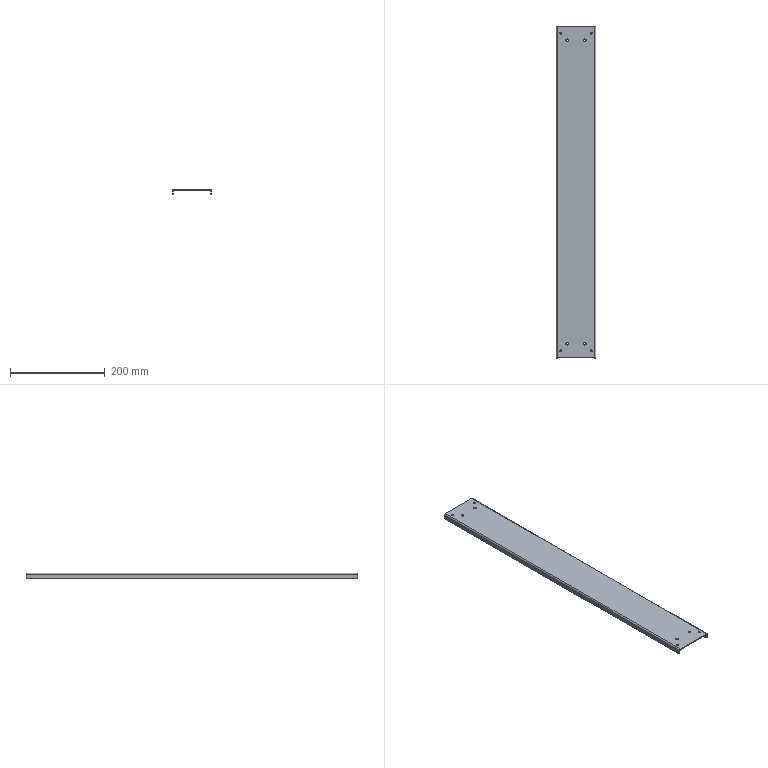Part | SolidWorks | features HoleWzd 3, Fillet 1, FlatPattern 1, SMBaseFlange 1, SheetMetal 1 | 1 solid | 42 faces | box 84 x 700 x 12 mm | volume 143164 mm3 | cylinder 24 | plane 18 | commonest cylinder face diameters 5.5 x10 4.5 x8 6 x4 1.5 x2
STEP:
#1=CARTESIAN_POINT('',(61.25,30.,2.));
#2=VERTEX_POINT('',#1);
#3=CARTESIAN_POINT('',(55.75,30.,2.));
#4=VERTEX_POINT('',#3);
#5=CARTESIAN_POINT('',(58.5,30.,2.));
#6=DIRECTION('',(0.,0.,-1.));
#7=DIRECTION('',(-1.,0.,0.));
#8=AXIS2_PLACEMENT_3D('',#5,#6,#7);
#9=CIRCLE('',#8,2.75);
#10=EDGE_CURVE('',#2,#4,#9,.T.);
#11=ORIENTED_EDGE('',*,*,#10,.F.);
#12=CARTESIAN_POINT('',(61.25,30.,0.));
#13=VERTEX_POINT('',#12);
#14=CARTESIAN_POINT('',(61.25,30.,0.));
#15=DIRECTION('',(0.,0.,-1.));
#16=VECTOR('',#15,1000.);
#17=LINE('',#14,#16);
#18=EDGE_CURVE('',#2,#13,#17,.T.);
#19=ORIENTED_EDGE('',*,*,#18,.T.);
#20=CARTESIAN_POINT('',(55.75,30.,0.));
#21=VERTEX_POINT('',#20);
#22=CARTESIAN_POINT('',(58.5,30.,0.));
#23=DIRECTION('',(0.,0.,-1.));
#24=DIRECTION('',(-1.,0.,0.));
#25=AXIS2_PLACEMENT_3D('',#22,#23,#24);
#26=CIRCLE('',#25,2.75);
#27=EDGE_CURVE('',#13,#21,#26,.T.);
#28=ORIENTED_EDGE('',*,*,#27,.T.);
#29=CARTESIAN_POINT('',(55.75,30.,0.));
#30=DIRECTION('',(0.,0.,-1.));
#31=VECTOR('',#30,1000.);
#32=LINE('',#29,#31);
#33=EDGE_CURVE('',#4,#21,#32,.T.);
#34=ORIENTED_EDGE('',*,*,#33,.F.);
#35=EDGE_LOOP('',(#11,#19,#28,#34));
#36=FACE_OUTER_BOUND('',#35,.T.);
#37=CARTESIAN_POINT('',(58.5,30.,0.));
#38=DIRECTION('',(0.,0.,-1.));
#39=DIRECTION('',(-1.,0.,0.));
#40=AXIS2_PLACEMENT_3D('',#37,#38,#39);
#41=CYLINDRICAL_SURFACE('',#40,2.75);
#42=ADVANCED_FACE('',(#36),#41,.F.);
#43=CARTESIAN_POINT('',(24.25,30.,2.));
#44=VERTEX_POINT('',#43);
#45=CARTESIAN_POINT('',(18.75,30.,2.));
#46=VERTEX_POINT('',#45);
#47=CARTESIAN_POINT('',(21.5,30.,2.));
#48=DIRECTION('',(0.,0.,-1.));
#49=DIRECTION('',(-1.,0.,0.));
#50=AXIS2_PLACEMENT_3D('',#47,#48,#49);
#51=CIRCLE('',#50,2.75);
#52=EDGE_CURVE('',#44,#46,#51,.T.);
#53=ORIENTED_EDGE('',*,*,#52,.F.);
#54=CARTESIAN_POINT('',(24.25,30.,0.));
#55=VERTEX_POINT('',#54);
#56=CARTESIAN_POINT('',(24.25,30.,0.));
#57=DIRECTION('',(0.,0.,-1.));
#58=VECTOR('',#57,1000.);
#59=LINE('',#56,#58);
#60=EDGE_CURVE('',#44,#55,#59,.T.);
#61=ORIENTED_EDGE('',*,*,#60,.T.);
#62=CARTESIAN_POINT('',(18.75,30.,0.));
#63=VERTEX_POINT('',#62);
#64=CARTESIAN_POINT('',(21.5,30.,0.));
#65=DIRECTION('',(0.,0.,-1.));
#66=DIRECTION('',(-1.,0.,0.));
#67=AXIS2_PLACEMENT_3D('',#64,#65,#66);
#68=CIRCLE('',#67,2.75);
#69=EDGE_CURVE('',#55,#63,#68,.T.);
#70=ORIENTED_EDGE('',*,*,#69,.T.);
#71=CARTESIAN_POINT('',(18.75,30.,0.));
#72=DIRECTION('',(0.,0.,-1.));
#73=VECTOR('',#72,1000.);
#74=LINE('',#71,#73);
#75=EDGE_CURVE('',#46,#63,#74,.T.);
#76=ORIENTED_EDGE('',*,*,#75,.F.);
#77=EDGE_LOOP('',(#53,#61,#70,#76));
#78=FACE_OUTER_BOUND('',#77,.T.);
#79=CARTESIAN_POINT('',(21.5,30.,0.));
#80=DIRECTION('',(0.,0.,-1.));
#81=DIRECTION('',(-1.,0.,0.));
#82=AXIS2_PLACEMENT_3D('',#79,#80,#81);
#83=CYLINDRICAL_SURFACE('',#82,2.75);
#84=ADVANCED_FACE('',(#78),#83,.F.);
#85=CARTESIAN_POINT('',(61.25,670.,2.));
#86=VERTEX_POINT('',#85);
#87=CARTESIAN_POINT('',(55.75,670.,2.));
#88=VERTEX_POINT('',#87);
#89=CARTESIAN_POINT('',(58.5,670.,2.));
#90=DIRECTION('',(0.,0.,-1.));
#91=DIRECTION('',(-1.,0.,0.));
#92=AXIS2_PLACEMENT_3D('',#89,#90,#91);
#93=CIRCLE('',#92,2.75);
#94=EDGE_CURVE('',#86,#88,#93,.T.);
#95=ORIENTED_EDGE('',*,*,#94,.F.);
#96=CARTESIAN_POINT('',(61.25,670.,0.));
#97=VERTEX_POINT('',#96);
#98=CARTESIAN_POINT('',(61.25,670.,0.));
#99=DIRECTION('',(0.,0.,-1.));
#100=VECTOR('',#99,1000.);
#101=LINE('',#98,#100);
#102=EDGE_CURVE('',#86,#97,#101,.T.);
#103=ORIENTED_EDGE('',*,*,#102,.T.);
#104=CARTESIAN_POINT('',(55.75,670.,0.));
#105=VERTEX_POINT('',#104);
#106=CARTESIAN_POINT('',(58.5,670.,0.));
#107=DIRECTION('',(0.,0.,-1.));
#108=DIRECTION('',(-1.,0.,0.));
#109=AXIS2_PLACEMENT_3D('',#106,#107,#108);
#110=CIRCLE('',#109,2.75);
#111=EDGE_CURVE('',#97,#105,#110,.T.);
#112=ORIENTED_EDGE('',*,*,#111,.T.);
#113=CARTESIAN_POINT('',(55.75,670.,0.));
#114=DIRECTION('',(0.,0.,-1.));
#115=VECTOR('',#114,1000.);
#116=LINE('',#113,#115);
#117=EDGE_CURVE('',#88,#105,#116,.T.);
#118=ORIENTED_EDGE('',*,*,#117,.F.);
#119=EDGE_LOOP('',(#95,#103,#112,#118));
#120=FACE_OUTER_BOUND('',#119,.T.);
#121=CARTESIAN_POINT('',(58.5,670.,0.));
#122=DIRECTION('',(0.,0.,-1.));
#123=DIRECTION('',(-1.,0.,0.));
#124=AXIS2_PLACEMENT_3D('',#121,#122,#123);
#125=CYLINDRICAL_SURFACE('',#124,2.75);
#126=ADVANCED_FACE('',(#120),#125,.F.);
#127=CARTESIAN_POINT('',(24.25,670.,2.));
#128=VERTEX_POINT('',#127);
#129=CARTESIAN_POINT('',(18.75,670.,2.));
#130=VERTEX_POINT('',#129);
#131=CARTESIAN_POINT('',(21.5,670.,2.));
#132=DIRECTION('',(0.,0.,-1.));
#133=DIRECTION('',(-1.,0.,0.));
#134=AXIS2_PLACEMENT_3D('',#131,#132,#133);
#135=CIRCLE('',#134,2.75);
#136=EDGE_CURVE('',#128,#130,#135,.T.);
#137=ORIENTED_EDGE('',*,*,#136,.F.);
#138=CARTESIAN_POINT('',(24.25,670.,0.));
#139=VERTEX_POINT('',#138);
#140=CARTESIAN_POINT('',(24.25,670.,0.));
#141=DIRECTION('',(0.,0.,-1.));
#142=VECTOR('',#141,1000.);
#143=LINE('',#140,#142);
#144=EDGE_CURVE('',#128,#139,#143,.T.);
#145=ORIENTED_EDGE('',*,*,#144,.T.);
#146=CARTESIAN_POINT('',(18.75,670.,0.));
#147=VERTEX_POINT('',#146);
#148=CARTESIAN_POINT('',(21.5,670.,0.));
#149=DIRECTION('',(0.,0.,-1.));
#150=DIRECTION('',(-1.,0.,0.));
#151=AXIS2_PLACEMENT_3D('',#148,#149,#150);
#152=CIRCLE('',#151,2.75);
#153=EDGE_CURVE('',#139,#147,#152,.T.);
#154=ORIENTED_EDGE('',*,*,#153,.T.);
#155=CARTESIAN_POINT('',(18.75,670.,0.));
#156=DIRECTION('',(0.,0.,-1.));
#157=VECTOR('',#156,1000.);
#158=LINE('',#155,#157);
#159=EDGE_CURVE('',#130,#147,#158,.T.);
#160=ORIENTED_EDGE('',*,*,#159,.F.);
#161=EDGE_LOOP('',(#137,#145,#154,#160));
#162=FACE_OUTER_BOUND('',#161,.T.);
#163=CARTESIAN_POINT('',(21.5,670.,0.));
#164=DIRECTION('',(0.,0.,-1.));
#165=DIRECTION('',(-1.,0.,0.));
#166=AXIS2_PLACEMENT_3D('',#163,#164,#165);
#167=CYLINDRICAL_SURFACE('',#166,2.75);
#168=ADVANCED_FACE('',(#162),#167,.F.);
#169=CARTESIAN_POINT('',(74.25,15.,2.));
#170=VERTEX_POINT('',#169);
#171=CARTESIAN_POINT('',(69.75,15.,2.));
#172=VERTEX_POINT('',#171);
#173=CARTESIAN_POINT('',(72.,15.,2.));
#174=DIRECTION('',(0.,0.,-1.));
#175=DIRECTION('',(-1.,0.,0.));
#176=AXIS2_PLACEMENT_3D('',#173,#174,#175);
#177=CIRCLE('',#176,2.25);
#178=EDGE_CURVE('',#170,#172,#177,.T.);
#179=ORIENTED_EDGE('',*,*,#178,.F.);
#180=CARTESIAN_POINT('',(74.25,15.,0.));
#181=VERTEX_POINT('',#180);
#182=CARTESIAN_POINT('',(74.25,15.,0.));
#183=DIRECTION('',(0.,0.,-1.));
#184=VECTOR('',#183,1000.);
#185=LINE('',#182,#184);
#186=EDGE_CURVE('',#170,#181,#185,.T.);
#187=ORIENTED_EDGE('',*,*,#186,.T.);
#188=CARTESIAN_POINT('',(69.75,15.,0.));
#189=VERTEX_POINT('',#188);
#190=CARTESIAN_POINT('',(72.,15.,0.));
#191=DIRECTION('',(0.,0.,-1.));
#192=DIRECTION('',(-1.,0.,0.));
#193=AXIS2_PLACEMENT_3D('',#190,#191,#192);
#194=CIRCLE('',#193,2.25);
#195=EDGE_CURVE('',#181,#189,#194,.T.);
#196=ORIENTED_EDGE('',*,*,#195,.T.);
#197=CARTESIAN_POINT('',(69.75,15.,0.));
#198=DIRECTION('',(0.,0.,-1.));
#199=VECTOR('',#198,1000.);
#200=LINE('',#197,#199);
#201=EDGE_CURVE('',#172,#189,#200,.T.);
#202=ORIENTED_EDGE('',*,*,#201,.F.);
#203=EDGE_LOOP('',(#179,#187,#196,#202));
#204=FACE_OUTER_BOUND('',#203,.T.);
#205=CARTESIAN_POINT('',(72.,15.,0.));
#206=DIRECTION('',(0.,0.,-1.));
#207=DIRECTION('',(-1.,0.,0.));
#208=AXIS2_PLACEMENT_3D('',#205,#206,#207);
#209=CYLINDRICAL_SURFACE('',#208,2.25);
#210=ADVANCED_FACE('',(#204),#209,.F.);
#211=CARTESIAN_POINT('',(74.25,685.,2.));
#212=VERTEX_POINT('',#211);
#213=CARTESIAN_POINT('',(69.75,685.,2.));
#214=VERTEX_POINT('',#213);
#215=CARTESIAN_POINT('',(72.,685.,2.));
#216=DIRECTION('',(0.,0.,-1.));
#217=DIRECTION('',(-1.,0.,0.));
#218=AXIS2_PLACEMENT_3D('',#215,#216,#217);
#219=CIRCLE('',#218,2.25);
#220=EDGE_CURVE('',#212,#214,#219,.T.);
#221=ORIENTED_EDGE('',*,*,#220,.F.);
#222=CARTESIAN_POINT('',(74.25,685.,0.));
#223=VERTEX_POINT('',#222);
#224=CARTESIAN_POINT('',(74.25,685.,0.));
#225=DIRECTION('',(0.,0.,-1.));
#226=VECTOR('',#225,1000.);
#227=LINE('',#224,#226);
#228=EDGE_CURVE('',#212,#223,#227,.T.);
#229=ORIENTED_EDGE('',*,*,#228,.T.);
#230=CARTESIAN_POINT('',(69.75,685.,0.));
#231=VERTEX_POINT('',#230);
#232=CARTESIAN_POINT('',(72.,685.,0.));
#233=DIRECTION('',(0.,0.,-1.));
#234=DIRECTION('',(-1.,0.,0.));
#235=AXIS2_PLACEMENT_3D('',#232,#233,#234);
#236=CIRCLE('',#235,2.25);
#237=EDGE_CURVE('',#223,#231,#236,.T.);
#238=ORIENTED_EDGE('',*,*,#237,.T.);
#239=CARTESIAN_POINT('',(69.75,685.,0.));
#240=DIRECTION('',(0.,0.,-1.));
#241=VECTOR('',#240,1000.);
#242=LINE('',#239,#241);
#243=EDGE_CURVE('',#214,#231,#242,.T.);
#244=ORIENTED_EDGE('',*,*,#243,.F.);
#245=EDGE_LOOP('',(#221,#229,#238,#244));
#246=FACE_OUTER_BOUND('',#245,.T.);
#247=CARTESIAN_POINT('',(72.,685.,0.));
#248=DIRECTION('',(0.,0.,-1.));
#249=DIRECTION('',(-1.,0.,0.));
#250=AXIS2_PLACEMENT_3D('',#247,#248,#249);
#251=CYLINDRICAL_SURFACE('',#250,2.25);
#252=ADVANCED_FACE('',(#246),#251,.F.);
#253=CARTESIAN_POINT('',(10.25,15.,2.));
#254=VERTEX_POINT('',#253);
#255=CARTESIAN_POINT('',(5.75,15.,2.));
#256=VERTEX_POINT('',#255);
#257=CARTESIAN_POINT('',(8.,15.,2.));
#258=DIRECTION('',(0.,0.,-1.));
#259=DIRECTION('',(-1.,0.,0.));
#260=AXIS2_PLACEMENT_3D('',#257,#258,#259);
#261=CIRCLE('',#260,2.25);
#262=EDGE_CURVE('',#254,#256,#261,.T.);
#263=ORIENTED_EDGE('',*,*,#262,.F.);
#264=CARTESIAN_POINT('',(10.25,15.,0.));
#265=VERTEX_POINT('',#264);
#266=CARTESIAN_POINT('',(10.25,15.,0.));
#267=DIRECTION('',(0.,0.,-1.));
#268=VECTOR('',#267,1000.);
#269=LINE('',#266,#268);
#270=EDGE_CURVE('',#254,#265,#269,.T.);
#271=ORIENTED_EDGE('',*,*,#270,.T.);
#272=CARTESIAN_POINT('',(5.75,15.,0.));
#273=VERTEX_POINT('',#272);
#274=CARTESIAN_POINT('',(8.,15.,0.));
#275=DIRECTION('',(0.,0.,-1.));
#276=DIRECTION('',(-1.,0.,0.));
#277=AXIS2_PLACEMENT_3D('',#274,#275,#276);
#278=CIRCLE('',#277,2.25);
#279=EDGE_CURVE('',#265,#273,#278,.T.);
#280=ORIENTED_EDGE('',*,*,#279,.T.);
#281=CARTESIAN_POINT('',(5.75,15.,0.));
#282=DIRECTION('',(0.,0.,-1.));
#283=VECTOR('',#282,1000.);
#284=LINE('',#281,#283);
#285=EDGE_CURVE('',#256,#273,#284,.T.);
#286=ORIENTED_EDGE('',*,*,#285,.F.);
#287=EDGE_LOOP('',(#263,#271,#280,#286));
#288=FACE_OUTER_BOUND('',#287,.T.);
#289=CARTESIAN_POINT('',(8.,15.,0.));
#290=DIRECTION('',(0.,0.,-1.));
#291=DIRECTION('',(-1.,0.,0.));
#292=AXIS2_PLACEMENT_3D('',#289,#290,#291);
#293=CYLINDRICAL_SURFACE('',#292,2.25);
#294=ADVANCED_FACE('',(#288),#293,.F.);
#295=CARTESIAN_POINT('',(10.25,685.,2.));
#296=VERTEX_POINT('',#295);
#297=CARTESIAN_POINT('',(5.75,685.,2.));
#298=VERTEX_POINT('',#297);
#299=CARTESIAN_POINT('',(8.,685.,2.));
#300=DIRECTION('',(0.,0.,-1.));
#301=DIRECTION('',(-1.,0.,0.));
#302=AXIS2_PLACEMENT_3D('',#299,#300,#301);
#303=CIRCLE('',#302,2.25);
#304=EDGE_CURVE('',#296,#298,#303,.T.);
#305=ORIENTED_EDGE('',*,*,#304,.F.);
#306=CARTESIAN_POINT('',(10.25,685.,0.));
#307=VERTEX_POINT('',#306);
#308=CARTESIAN_POINT('',(10.25,685.,0.));
#309=DIRECTION('',(0.,0.,-1.));
#310=VECTOR('',#309,1000.);
#311=LINE('',#308,#310);
#312=EDGE_CURVE('',#296,#307,#311,.T.);
#313=ORIENTED_EDGE('',*,*,#312,.T.);
#314=CARTESIAN_POINT('',(5.75,685.,0.));
#315=VERTEX_POINT('',#314);
#316=CARTESIAN_POINT('',(8.,685.,0.));
#317=DIRECTION('',(0.,0.,-1.));
#318=DIRECTION('',(-1.,0.,0.));
#319=AXIS2_PLACEMENT_3D('',#316,#317,#318);
#320=CIRCLE('',#319,2.25);
#321=EDGE_CURVE('',#307,#315,#320,.T.);
#322=ORIENTED_EDGE('',*,*,#321,.T.);
#323=CARTESIAN_POINT('',(5.75,685.,0.));
#324=DIRECTION('',(0.,0.,-1.));
#325=VECTOR('',#324,1000.);
#326=LINE('',#323,#325);
#327=EDGE_CURVE('',#298,#315,#326,.T.);
#328=ORIENTED_EDGE('',*,*,#327,.F.);
#329=EDGE_LOOP('',(#305,#313,#322,#328));
#330=FACE_OUTER_BOUND('',#329,.T.);
#331=CARTESIAN_POINT('',(8.,685.,0.));
#332=DIRECTION('',(0.,0.,-1.));
#333=DIRECTION('',(-1.,0.,0.));
#334=AXIS2_PLACEMENT_3D('',#331,#332,#333);
#335=CYLINDRICAL_SURFACE('',#334,2.25);
#336=ADVANCED_FACE('',(#330),#335,.F.);
#337=CARTESIAN_POINT('',(0.75,700.,0.));
#338=VERTEX_POINT('',#337);
#339=CARTESIAN_POINT('',(0.75,700.,2.));
#340=VERTEX_POINT('',#339);
#341=CARTESIAN_POINT('',(0.75,700.,0.));
#342=DIRECTION('',(0.,0.,1.));
#343=VECTOR('',#342,1000.);
#344=LINE('',#341,#343);
#345=EDGE_CURVE('',#338,#340,#344,.T.);
#346=ORIENTED_EDGE('',*,*,#345,.F.);
#347=CARTESIAN_POINT('',(0.,700.,-0.75));
#348=VERTEX_POINT('',#347);
#349=CARTESIAN_POINT('',(0.75,700.,-0.75));
#350=DIRECTION('',(0.,1.,0.));
#351=DIRECTION('',(0.,0.,-1.));
#352=AXIS2_PLACEMENT_3D('',#349,#350,#351);
#353=CIRCLE('',#352,0.75);
#354=EDGE_CURVE('',#348,#338,#353,.T.);
#355=ORIENTED_EDGE('',*,*,#354,.F.);
#356=CARTESIAN_POINT('',(-2.,700.,-0.75));
#357=VERTEX_POINT('',#356);
#358=CARTESIAN_POINT('',(-2.,700.,-0.75));
#359=DIRECTION('',(1.,0.,0.));
#360=VECTOR('',#359,1000.);
#361=LINE('',#358,#360);
#362=EDGE_CURVE('',#357,#348,#361,.T.);
#363=ORIENTED_EDGE('',*,*,#362,.F.);
#364=CARTESIAN_POINT('',(0.75,700.,-0.75));
#365=DIRECTION('',(0.,1.,0.));
#366=DIRECTION('',(1.,0.,0.));
#367=AXIS2_PLACEMENT_3D('',#364,#365,#366);
#368=CIRCLE('',#367,2.75);
#369=EDGE_CURVE('',#357,#340,#368,.T.);
#370=ORIENTED_EDGE('',*,*,#369,.T.);
#371=EDGE_LOOP('',(#346,#355,#363,#370));
#372=FACE_OUTER_BOUND('',#371,.T.);
#373=CARTESIAN_POINT('',(0.75,700.,0.));
#374=DIRECTION('',(0.,1.,0.));
#375=DIRECTION('',(0.,0.,1.));
#376=AXIS2_PLACEMENT_3D('',#373,#374,#375);
#377=PLANE('',#376);
#378=ADVANCED_FACE('',(#372),#377,.T.);
#379=CARTESIAN_POINT('',(79.25,700.,0.));
#380=VERTEX_POINT('',#379);
#381=CARTESIAN_POINT('',(0.,700.,0.));
#382=DIRECTION('',(1.,0.,0.));
#383=VECTOR('',#382,1000.);
#384=LINE('',#381,#383);
#385=EDGE_CURVE('',#338,#380,#384,.T.);
#386=ORIENTED_EDGE('',*,*,#385,.F.);
#387=ORIENTED_EDGE('',*,*,#345,.T.);
#388=CARTESIAN_POINT('',(79.25,700.,2.));
#389=VERTEX_POINT('',#388);
#390=CARTESIAN_POINT('',(0.,700.,2.));
#391=DIRECTION('',(1.,0.,0.));
#392=VECTOR('',#391,1000.);
#393=LINE('',#390,#392);
#394=EDGE_CURVE('',#340,#389,#393,.T.);
#395=ORIENTED_EDGE('',*,*,#394,.T.);
#396=CARTESIAN_POINT('',(79.25,700.,2.));
#397=DIRECTION('',(0.,0.,-1.));
#398=VECTOR('',#397,1000.);
#399=LINE('',#396,#398);
#400=EDGE_CURVE('',#389,#380,#399,.T.);
#401=ORIENTED_EDGE('',*,*,#400,.T.);
#402=EDGE_LOOP('',(#386,#387,#395,#401));
#403=FACE_OUTER_BOUND('',#402,.T.);
#404=CARTESIAN_POINT('',(-2.,700.,-0.75));
#405=DIRECTION('',(0.,1.,0.));
#406=DIRECTION('',(0.,0.,1.));
#407=AXIS2_PLACEMENT_3D('',#404,#405,#406);
#408=PLANE('',#407);
#409=ADVANCED_FACE('',(#403),#408,.T.);
#410=CARTESIAN_POINT('',(0.,0.,-0.75));
#411=VERTEX_POINT('',#410);
#412=CARTESIAN_POINT('',(-2.,0.,-0.75));
#413=VERTEX_POINT('',#412);
#414=CARTESIAN_POINT('',(0.,0.,-0.75));
#415=DIRECTION('',(-1.,0.,0.));
#416=VECTOR('',#415,1000.);
#417=LINE('',#414,#416);
#418=EDGE_CURVE('',#411,#413,#417,.T.);
#419=ORIENTED_EDGE('',*,*,#418,.F.);
#420=CARTESIAN_POINT('',(0.75,0.,0.));
#421=VERTEX_POINT('',#420);
#422=CARTESIAN_POINT('',(0.75,0.,-0.75));
#423=DIRECTION('',(0.,1.,0.));
#424=DIRECTION('',(0.,0.,-1.));
#425=AXIS2_PLACEMENT_3D('',#422,#423,#424);
#426=CIRCLE('',#425,0.75);
#427=EDGE_CURVE('',#411,#421,#426,.T.);
#428=ORIENTED_EDGE('',*,*,#427,.T.);
#429=CARTESIAN_POINT('',(0.75,0.,2.));
#430=VERTEX_POINT('',#429);
#431=CARTESIAN_POINT('',(0.75,0.,2.));
#432=DIRECTION('',(0.,0.,-1.));
#433=VECTOR('',#432,1000.);
#434=LINE('',#431,#433);
#435=EDGE_CURVE('',#430,#421,#434,.T.);
#436=ORIENTED_EDGE('',*,*,#435,.F.);
#437=CARTESIAN_POINT('',(0.75,0.,-0.75));
#438=DIRECTION('',(0.,1.,0.));
#439=DIRECTION('',(1.,0.,0.));
#440=AXIS2_PLACEMENT_3D('',#437,#438,#439);
#441=CIRCLE('',#440,2.75);
#442=EDGE_CURVE('',#413,#430,#441,.T.);
#443=ORIENTED_EDGE('',*,*,#442,.F.);
#444=EDGE_LOOP('',(#419,#428,#436,#443));
#445=FACE_OUTER_BOUND('',#444,.T.);
#446=CARTESIAN_POINT('',(0.,0.,-0.75));
#447=DIRECTION('',(0.,-1.,0.));
#448=DIRECTION('',(0.,0.,-1.));
#449=AXIS2_PLACEMENT_3D('',#446,#447,#448);
#450=PLANE('',#449);
#451=ADVANCED_FACE('',(#445),#450,.T.);
#452=CARTESIAN_POINT('',(-2.,0.,-7.));
#453=VERTEX_POINT('',#452);
#454=CARTESIAN_POINT('',(-2.,0.,-10.));
#455=DIRECTION('',(0.,0.,1.));
#456=VECTOR('',#455,1000.);
#457=LINE('',#454,#456);
#458=EDGE_CURVE('',#453,#413,#457,.T.);
#459=ORIENTED_EDGE('',*,*,#458,.F.);
#460=CARTESIAN_POINT('',(0.,0.,-7.));
#461=VERTEX_POINT('',#460);
#462=CARTESIAN_POINT('',(0.75,0.,-7.));
#463=DIRECTION('',(1.,0.,0.));
#464=VECTOR('',#463,1000.);
#465=LINE('',#462,#464);
#466=EDGE_CURVE('',#453,#461,#465,.T.);
#467=ORIENTED_EDGE('',*,*,#466,.T.);
#468=CARTESIAN_POINT('',(0.,0.,-10.));
#469=DIRECTION('',(0.,0.,1.));
#470=VECTOR('',#469,1000.);
#471=LINE('',#468,#470);
#472=EDGE_CURVE('',#461,#411,#471,.T.);
#473=ORIENTED_EDGE('',*,*,#472,.T.);
#474=ORIENTED_EDGE('',*,*,#418,.T.);
#475=EDGE_LOOP('',(#459,#467,#473,#474));
#476=FACE_OUTER_BOUND('',#475,.T.);
#477=CARTESIAN_POINT('',(0.75,0.,2.));
#478=DIRECTION('',(0.,-1.,0.));
#479=DIRECTION('',(0.,0.,-1.));
#480=AXIS2_PLACEMENT_3D('',#477,#478,#479);
#481=PLANE('',#480);
#482=ADVANCED_FACE('',(#476),#481,.T.);
#483=CARTESIAN_POINT('',(80.,700.,-0.75));
#484=VERTEX_POINT('',#483);
#485=CARTESIAN_POINT('',(82.,700.,-0.75));
#486=VERTEX_POINT('',#485);
#487=CARTESIAN_POINT('',(80.,700.,-0.75));
#488=DIRECTION('',(1.,0.,0.));
#489=VECTOR('',#488,1000.);
#490=LINE('',#487,#489);
#491=EDGE_CURVE('',#484,#486,#490,.T.);
#492=ORIENTED_EDGE('',*,*,#491,.F.);
#493=CARTESIAN_POINT('',(79.25,700.,-0.75));
#494=DIRECTION('',(0.,1.,0.));
#495=DIRECTION('',(0.,0.,-1.));
#496=AXIS2_PLACEMENT_3D('',#493,#494,#495);
#497=CIRCLE('',#496,0.75);
#498=EDGE_CURVE('',#380,#484,#497,.T.);
#499=ORIENTED_EDGE('',*,*,#498,.F.);
#500=ORIENTED_EDGE('',*,*,#400,.F.);
#501=CARTESIAN_POINT('',(79.25,700.,-0.75));
#502=DIRECTION('',(0.,1.,0.));
#503=DIRECTION('',(1.,0.,0.));
#504=AXIS2_PLACEMENT_3D('',#501,#502,#503);
#505=CIRCLE('',#504,2.75);
#506=EDGE_CURVE('',#389,#486,#505,.T.);
#507=ORIENTED_EDGE('',*,*,#506,.T.);
#508=EDGE_LOOP('',(#492,#499,#500,#507));
#509=FACE_OUTER_BOUND('',#508,.T.);
#510=CARTESIAN_POINT('',(80.,700.,-0.75));
#511=DIRECTION('',(0.,1.,0.));
#512=DIRECTION('',(0.,0.,1.));
#513=AXIS2_PLACEMENT_3D('',#510,#511,#512);
#514=PLANE('',#513);
#515=ADVANCED_FACE('',(#509),#514,.T.);
#516=CARTESIAN_POINT('',(82.,700.,-7.));
#517=VERTEX_POINT('',#516);
#518=CARTESIAN_POINT('',(82.,700.,0.));
#519=DIRECTION('',(0.,0.,-1.));
#520=VECTOR('',#519,1000.);
#521=LINE('',#518,#520);
#522=EDGE_CURVE('',#486,#517,#521,.T.);
#523=ORIENTED_EDGE('',*,*,#522,.T.);
#524=CARTESIAN_POINT('',(80.,700.,-7.));
#525=VERTEX_POINT('',#524);
#526=CARTESIAN_POINT('',(79.25,700.,-7.));
#527=DIRECTION('',(-1.,0.,0.));
#528=VECTOR('',#527,1000.);
#529=LINE('',#526,#528);
#530=EDGE_CURVE('',#517,#525,#529,.T.);
#531=ORIENTED_EDGE('',*,*,#530,.T.);
#532=CARTESIAN_POINT('',(80.,700.,0.));
#533=DIRECTION('',(0.,0.,-1.));
#534=VECTOR('',#533,1000.);
#535=LINE('',#532,#534);
#536=EDGE_CURVE('',#484,#525,#535,.T.);
#537=ORIENTED_EDGE('',*,*,#536,.F.);
#538=ORIENTED_EDGE('',*,*,#491,.T.);
#539=EDGE_LOOP('',(#523,#531,#537,#538));
#540=FACE_OUTER_BOUND('',#539,.T.);
#541=CARTESIAN_POINT('',(79.25,700.,2.));
#542=DIRECTION('',(0.,1.,0.));
#543=DIRECTION('',(0.,0.,1.));
#544=AXIS2_PLACEMENT_3D('',#541,#542,#543);
#545=PLANE('',#544);
#546=ADVANCED_FACE('',(#540),#545,.T.);
#547=CARTESIAN_POINT('',(79.25,0.,0.));
#548=VERTEX_POINT('',#547);
#549=CARTESIAN_POINT('',(79.25,0.,2.));
#550=VERTEX_POINT('',#549);
#551=CARTESIAN_POINT('',(79.25,0.,0.));
#552=DIRECTION('',(0.,0.,1.));
#553=VECTOR('',#552,1000.);
#554=LINE('',#551,#553);
#555=EDGE_CURVE('',#548,#550,#554,.T.);
#556=ORIENTED_EDGE('',*,*,#555,.F.);
#557=CARTESIAN_POINT('',(80.,0.,-0.75));
#558=VERTEX_POINT('',#557);
#559=CARTESIAN_POINT('',(79.25,0.,-0.75));
#560=DIRECTION('',(0.,1.,0.));
#561=DIRECTION('',(0.,0.,-1.));
#562=AXIS2_PLACEMENT_3D('',#559,#560,#561);
#563=CIRCLE('',#562,0.75);
#564=EDGE_CURVE('',#548,#558,#563,.T.);
#565=ORIENTED_EDGE('',*,*,#564,.T.);
#566=CARTESIAN_POINT('',(82.,0.,-0.75));
#567=VERTEX_POINT('',#566);
#568=CARTESIAN_POINT('',(82.,0.,-0.75));
#569=DIRECTION('',(-1.,0.,0.));
#570=VECTOR('',#569,1000.);
#571=LINE('',#568,#570);
#572=EDGE_CURVE('',#567,#558,#571,.T.);
#573=ORIENTED_EDGE('',*,*,#572,.F.);
#574=CARTESIAN_POINT('',(79.25,0.,-0.75));
#575=DIRECTION('',(0.,1.,0.));
#576=DIRECTION('',(1.,0.,0.));
#577=AXIS2_PLACEMENT_3D('',#574,#575,#576);
#578=CIRCLE('',#577,2.75);
#579=EDGE_CURVE('',#550,#567,#578,.T.);
#580=ORIENTED_EDGE('',*,*,#579,.F.);
#581=EDGE_LOOP('',(#556,#565,#573,#580));
#582=FACE_OUTER_BOUND('',#581,.T.);
#583=CARTESIAN_POINT('',(79.25,0.,0.));
#584=DIRECTION('',(0.,-1.,0.));
#585=DIRECTION('',(0.,0.,-1.));
#586=AXIS2_PLACEMENT_3D('',#583,#584,#585);
#587=PLANE('',#586);
#588=ADVANCED_FACE('',(#582),#587,.T.);
#589=CARTESIAN_POINT('',(0.,0.,0.));
#590=DIRECTION('',(1.,0.,0.));
#591=VECTOR('',#590,1000.);
#592=LINE('',#589,#591);
#593=EDGE_CURVE('',#421,#548,#592,.T.);
#594=ORIENTED_EDGE('',*,*,#593,.T.);
#595=ORIENTED_EDGE('',*,*,#555,.T.);
#596=CARTESIAN_POINT('',(0.,0.,2.));
#597=DIRECTION('',(1.,0.,0.));
#598=VECTOR('',#597,1000.);
#599=LINE('',#596,#598);
#600=EDGE_CURVE('',#430,#550,#599,.T.);
#601=ORIENTED_EDGE('',*,*,#600,.F.);
#602=ORIENTED_EDGE('',*,*,#435,.T.);
#603=EDGE_LOOP('',(#594,#595,#601,#602));
#604=FACE_OUTER_BOUND('',#603,.T.);
#605=CARTESIAN_POINT('',(82.,0.,-0.75));
#606=DIRECTION('',(0.,-1.,0.));
#607=DIRECTION('',(0.,0.,-1.));
#608=AXIS2_PLACEMENT_3D('',#605,#606,#607);
#609=PLANE('',#608);
#610=ADVANCED_FACE('',(#604),#609,.T.);
#611=CARTESIAN_POINT('',(82.,697.,-10.));
#612=VERTEX_POINT('',#611);
#613=CARTESIAN_POINT('',(82.,3.,-10.));
#614=VERTEX_POINT('',#613);
#615=CARTESIAN_POINT('',(82.,700.,-10.));
#616=DIRECTION('',(0.,-1.,0.));
#617=VECTOR('',#616,1000.);
#618=LINE('',#615,#617);
#619=EDGE_CURVE('',#612,#614,#618,.T.);
#620=ORIENTED_EDGE('',*,*,#619,.F.);
#621=CARTESIAN_POINT('',(82.,697.,-7.));
#622=DIRECTION('',(1.,0.,0.));
#623=DIRECTION('',(0.,0.,1.));
#624=AXIS2_PLACEMENT_3D('',#621,#622,#623);
#625=CIRCLE('',#624,3.);
#626=EDGE_CURVE('',#612,#517,#625,.T.);
#627=ORIENTED_EDGE('',*,*,#626,.T.);
#628=ORIENTED_EDGE('',*,*,#522,.F.);
#629=CARTESIAN_POINT('',(82.,700.,-0.75));
#630=DIRECTION('',(0.,-1.,0.));
#631=VECTOR('',#630,1000.);
#632=LINE('',#629,#631);
#633=EDGE_CURVE('',#486,#567,#632,.T.);
#634=ORIENTED_EDGE('',*,*,#633,.T.);
#635=CARTESIAN_POINT('',(82.,0.,-7.));
#636=VERTEX_POINT('',#635);
#637=CARTESIAN_POINT('',(82.,0.,0.));
#638=DIRECTION('',(0.,0.,-1.));
#639=VECTOR('',#638,1000.);
#640=LINE('',#637,#639);
#641=EDGE_CURVE('',#567,#636,#640,.T.);
#642=ORIENTED_EDGE('',*,*,#641,.T.);
#643=CARTESIAN_POINT('',(82.,3.,-7.));
#644=DIRECTION('',(1.,0.,0.));
#645=DIRECTION('',(0.,0.,1.));
#646=AXIS2_PLACEMENT_3D('',#643,#644,#645);
#647=CIRCLE('',#646,3.);
#648=EDGE_CURVE('',#636,#614,#647,.T.);
#649=ORIENTED_EDGE('',*,*,#648,.T.);
#650=EDGE_LOOP('',(#620,#627,#628,#634,#642,#649));
#651=FACE_OUTER_BOUND('',#650,.T.);
#652=CARTESIAN_POINT('',(82.,700.,0.));
#653=DIRECTION('',(-1.,0.,0.));
#654=DIRECTION('',(0.,0.,1.));
#655=AXIS2_PLACEMENT_3D('',#652,#653,#654);
#656=PLANE('',#655);
#657=ADVANCED_FACE('',(#651),#656,.F.);
#658=CARTESIAN_POINT('',(80.,697.,-10.));
#659=VERTEX_POINT('',#658);
#660=CARTESIAN_POINT('',(80.,3.,-10.));
#661=VERTEX_POINT('',#660);
#662=CARTESIAN_POINT('',(80.,700.,-10.));
#663=DIRECTION('',(0.,-1.,0.));
#664=VECTOR('',#663,1000.);
#665=LINE('',#662,#664);
#666=EDGE_CURVE('',#659,#661,#665,.T.);
#667=ORIENTED_EDGE('',*,*,#666,.F.);
#668=CARTESIAN_POINT('',(80.,697.,-10.));
#669=DIRECTION('',(1.,0.,0.));
#670=VECTOR('',#669,1000.);
#671=LINE('',#668,#670);
#672=EDGE_CURVE('',#659,#612,#671,.T.);
#673=ORIENTED_EDGE('',*,*,#672,.T.);
#674=ORIENTED_EDGE('',*,*,#619,.T.);
#675=CARTESIAN_POINT('',(80.,3.,-10.));
#676=DIRECTION('',(-1.,0.,0.));
#677=VECTOR('',#676,1000.);
#678=LINE('',#675,#677);
#679=EDGE_CURVE('',#614,#661,#678,.T.);
#680=ORIENTED_EDGE('',*,*,#679,.T.);
#681=EDGE_LOOP('',(#667,#673,#674,#680));
#682=FACE_OUTER_BOUND('',#681,.T.);
#683=CARTESIAN_POINT('',(80.,700.,-10.));
#684=DIRECTION('',(0.,0.,-1.));
#685=DIRECTION('',(-1.,0.,0.));
#686=AXIS2_PLACEMENT_3D('',#683,#684,#685);
#687=PLANE('',#686);
#688=ADVANCED_FACE('',(#682),#687,.T.);
#689=ORIENTED_EDGE('',*,*,#536,.T.);
#690=CARTESIAN_POINT('',(80.,697.,-7.));
#691=DIRECTION('',(-1.,0.,0.));
#692=DIRECTION('',(0.,0.,1.));
#693=AXIS2_PLACEMENT_3D('',#690,#691,#692);
#694=CIRCLE('',#693,3.);
#695=EDGE_CURVE('',#525,#659,#694,.T.);
#696=ORIENTED_EDGE('',*,*,#695,.T.);
#697=ORIENTED_EDGE('',*,*,#666,.T.);
#698=CARTESIAN_POINT('',(80.,0.,-7.));
#699=VERTEX_POINT('',#698);
#700=CARTESIAN_POINT('',(80.,3.,-7.));
#701=DIRECTION('',(-1.,0.,0.));
#702=DIRECTION('',(0.,0.,1.));
#703=AXIS2_PLACEMENT_3D('',#700,#701,#702);
#704=CIRCLE('',#703,3.);
#705=EDGE_CURVE('',#661,#699,#704,.T.);
#706=ORIENTED_EDGE('',*,*,#705,.T.);
#707=CARTESIAN_POINT('',(80.,0.,0.));
#708=DIRECTION('',(0.,0.,-1.));
#709=VECTOR('',#708,1000.);
#710=LINE('',#707,#709);
#711=EDGE_CURVE('',#558,#699,#710,.T.);
#712=ORIENTED_EDGE('',*,*,#711,.F.);
#713=CARTESIAN_POINT('',(80.,700.,-0.75));
#714=DIRECTION('',(0.,-1.,0.));
#715=VECTOR('',#714,1000.);
#716=LINE('',#713,#715);
#717=EDGE_CURVE('',#484,#558,#716,.T.);
#718=ORIENTED_EDGE('',*,*,#717,.F.);
#719=EDGE_LOOP('',(#689,#696,#697,#706,#712,#718));
#720=FACE_OUTER_BOUND('',#719,.T.);
#721=CARTESIAN_POINT('',(80.,700.,0.));
#722=DIRECTION('',(-1.,0.,0.));
#723=DIRECTION('',(0.,0.,1.));
#724=AXIS2_PLACEMENT_3D('',#721,#722,#723);
#725=PLANE('',#724);
#726=ADVANCED_FACE('',(#720),#725,.T.);
#727=ORIENTED_EDGE('',*,*,#564,.F.);
#728=CARTESIAN_POINT('',(79.25,700.,0.));
#729=DIRECTION('',(0.,-1.,0.));
#730=VECTOR('',#729,1000.);
#731=LINE('',#728,#730);
#732=EDGE_CURVE('',#380,#548,#731,.T.);
#733=ORIENTED_EDGE('',*,*,#732,.F.);
#734=ORIENTED_EDGE('',*,*,#498,.T.);
#735=ORIENTED_EDGE('',*,*,#717,.T.);
#736=EDGE_LOOP('',(#727,#733,#734,#735));
#737=FACE_OUTER_BOUND('',#736,.T.);
#738=CARTESIAN_POINT('',(79.25,700.,-0.75));
#739=DIRECTION('',(0.,-1.,0.));
#740=DIRECTION('',(0.,0.,-1.));
#741=AXIS2_PLACEMENT_3D('',#738,#739,#740);
#742=CYLINDRICAL_SURFACE('',#741,0.75);
#743=ADVANCED_FACE('',(#737),#742,.F.);
#744=CARTESIAN_POINT('',(58.5,30.,0.));
#745=DIRECTION('',(0.,0.,-1.));
#746=DIRECTION('',(-1.,0.,0.));
#747=AXIS2_PLACEMENT_3D('',#744,#745,#746);
#748=CIRCLE('',#747,2.75);
#749=EDGE_CURVE('',#21,#13,#748,.T.);
#750=ORIENTED_EDGE('',*,*,#749,.F.);
#751=ORIENTED_EDGE('',*,*,#27,.F.);
#752=EDGE_LOOP('',(#750,#751));
#753=FACE_BOUND('',#752,.T.);
#754=CARTESIAN_POINT('',(21.5,30.,0.));
#755=DIRECTION('',(0.,0.,-1.));
#756=DIRECTION('',(-1.,0.,0.));
#757=AXIS2_PLACEMENT_3D('',#754,#755,#756);
#758=CIRCLE('',#757,2.75);
#759=EDGE_CURVE('',#63,#55,#758,.T.);
#760=ORIENTED_EDGE('',*,*,#759,.F.);
#761=ORIENTED_EDGE('',*,*,#69,.F.);
#762=EDGE_LOOP('',(#760,#761));
#763=FACE_BOUND('',#762,.T.);
#764=CARTESIAN_POINT('',(58.5,670.,0.));
#765=DIRECTION('',(0.,0.,-1.));
#766=DIRECTION('',(-1.,0.,0.));
#767=AXIS2_PLACEMENT_3D('',#764,#765,#766);
#768=CIRCLE('',#767,2.75);
#769=EDGE_CURVE('',#105,#97,#768,.T.);
#770=ORIENTED_EDGE('',*,*,#769,.F.);
#771=ORIENTED_EDGE('',*,*,#111,.F.);
#772=EDGE_LOOP('',(#770,#771));
#773=FACE_BOUND('',#772,.T.);
#774=CARTESIAN_POINT('',(21.5,670.,0.));
#775=DIRECTION('',(0.,0.,-1.));
#776=DIRECTION('',(-1.,0.,0.));
#777=AXIS2_PLACEMENT_3D('',#774,#775,#776);
#778=CIRCLE('',#777,2.75);
#779=EDGE_CURVE('',#147,#139,#778,.T.);
#780=ORIENTED_EDGE('',*,*,#779,.F.);
#781=ORIENTED_EDGE('',*,*,#153,.F.);
#782=EDGE_LOOP('',(#780,#781));
#783=FACE_BOUND('',#782,.T.);
#784=CARTESIAN_POINT('',(72.,15.,0.));
#785=DIRECTION('',(0.,0.,-1.));
#786=DIRECTION('',(-1.,0.,0.));
#787=AXIS2_PLACEMENT_3D('',#784,#785,#786);
#788=CIRCLE('',#787,2.25);
#789=EDGE_CURVE('',#189,#181,#788,.T.);
#790=ORIENTED_EDGE('',*,*,#789,.F.);
#791=ORIENTED_EDGE('',*,*,#195,.F.);
#792=EDGE_LOOP('',(#790,#791));
#793=FACE_BOUND('',#792,.T.);
#794=CARTESIAN_POINT('',(72.,685.,0.));
#795=DIRECTION('',(0.,0.,-1.));
#796=DIRECTION('',(-1.,0.,0.));
#797=AXIS2_PLACEMENT_3D('',#794,#795,#796);
#798=CIRCLE('',#797,2.25);
#799=EDGE_CURVE('',#231,#223,#798,.T.);
#800=ORIENTED_EDGE('',*,*,#799,.F.);
#801=ORIENTED_EDGE('',*,*,#237,.F.);
#802=EDGE_LOOP('',(#800,#801));
#803=FACE_BOUND('',#802,.T.);
#804=CARTESIAN_POINT('',(8.,15.,0.));
#805=DIRECTION('',(0.,0.,-1.));
#806=DIRECTION('',(-1.,0.,0.));
#807=AXIS2_PLACEMENT_3D('',#804,#805,#806);
#808=CIRCLE('',#807,2.25);
#809=EDGE_CURVE('',#273,#265,#808,.T.);
#810=ORIENTED_EDGE('',*,*,#809,.F.);
#811=ORIENTED_EDGE('',*,*,#279,.F.);
#812=EDGE_LOOP('',(#810,#811));
#813=FACE_BOUND('',#812,.T.);
#814=CARTESIAN_POINT('',(8.,685.,0.));
#815=DIRECTION('',(0.,0.,-1.));
#816=DIRECTION('',(-1.,0.,0.));
#817=AXIS2_PLACEMENT_3D('',#814,#815,#816);
#818=CIRCLE('',#817,2.25);
#819=EDGE_CURVE('',#315,#307,#818,.T.);
#820=ORIENTED_EDGE('',*,*,#819,.F.);
#821=ORIENTED_EDGE('',*,*,#321,.F.);
#822=EDGE_LOOP('',(#820,#821));
#823=FACE_BOUND('',#822,.T.);
#824=ORIENTED_EDGE('',*,*,#593,.F.);
#825=CARTESIAN_POINT('',(0.75,700.,0.));
#826=DIRECTION('',(0.,-1.,0.));
#827=VECTOR('',#826,1000.);
#828=LINE('',#825,#827);
#829=EDGE_CURVE('',#338,#421,#828,.T.);
#830=ORIENTED_EDGE('',*,*,#829,.F.);
#831=ORIENTED_EDGE('',*,*,#385,.T.);
#832=ORIENTED_EDGE('',*,*,#732,.T.);
#833=EDGE_LOOP('',(#824,#830,#831,#832));
#834=FACE_OUTER_BOUND('',#833,.T.);
#835=CARTESIAN_POINT('',(0.,700.,0.));
#836=DIRECTION('',(0.,0.,-1.));
#837=DIRECTION('',(-1.,0.,0.));
#838=AXIS2_PLACEMENT_3D('',#835,#836,#837);
#839=PLANE('',#838);
#840=ADVANCED_FACE('',(#753,#763,#773,#783,#793,#803,#813,#823,#834),#839,.T.);
#841=ORIENTED_EDGE('',*,*,#427,.F.);
#842=CARTESIAN_POINT('',(0.,700.,-0.75));
#843=DIRECTION('',(0.,-1.,0.));
#844=VECTOR('',#843,1000.);
#845=LINE('',#842,#844);
#846=EDGE_CURVE('',#348,#411,#845,.T.);
#847=ORIENTED_EDGE('',*,*,#846,.F.);
#848=ORIENTED_EDGE('',*,*,#354,.T.);
#849=ORIENTED_EDGE('',*,*,#829,.T.);
#850=EDGE_LOOP('',(#841,#847,#848,#849));
#851=FACE_OUTER_BOUND('',#850,.T.);
#852=CARTESIAN_POINT('',(0.75,700.,-0.75));
#853=DIRECTION('',(0.,-1.,0.));
#854=DIRECTION('',(0.,0.,-1.));
#855=AXIS2_PLACEMENT_3D('',#852,#853,#854);
#856=CYLINDRICAL_SURFACE('',#855,0.75);
#857=ADVANCED_FACE('',(#851),#856,.F.);
#858=CARTESIAN_POINT('',(0.,697.,-10.));
#859=VERTEX_POINT('',#858);
#860=CARTESIAN_POINT('',(0.,3.,-10.));
#861=VERTEX_POINT('',#860);
#862=CARTESIAN_POINT('',(0.,700.,-10.));
#863=DIRECTION('',(0.,-1.,0.));
#864=VECTOR('',#863,1000.);
#865=LINE('',#862,#864);
#866=EDGE_CURVE('',#859,#861,#865,.T.);
#867=ORIENTED_EDGE('',*,*,#866,.F.);
#868=CARTESIAN_POINT('',(0.,700.,-7.));
#869=VERTEX_POINT('',#868);
#870=CARTESIAN_POINT('',(0.,697.,-7.));
#871=DIRECTION('',(1.,0.,0.));
#872=DIRECTION('',(0.,0.,-1.));
#873=AXIS2_PLACEMENT_3D('',#870,#871,#872);
#874=CIRCLE('',#873,3.);
#875=EDGE_CURVE('',#859,#869,#874,.T.);
#876=ORIENTED_EDGE('',*,*,#875,.T.);
#877=CARTESIAN_POINT('',(0.,700.,-10.));
#878=DIRECTION('',(0.,0.,1.));
#879=VECTOR('',#878,1000.);
#880=LINE('',#877,#879);
#881=EDGE_CURVE('',#869,#348,#880,.T.);
#882=ORIENTED_EDGE('',*,*,#881,.T.);
#883=ORIENTED_EDGE('',*,*,#846,.T.);
#884=ORIENTED_EDGE('',*,*,#472,.F.);
#885=CARTESIAN_POINT('',(0.,3.,-7.));
#886=DIRECTION('',(1.,0.,0.));
#887=DIRECTION('',(0.,0.,-1.));
#888=AXIS2_PLACEMENT_3D('',#885,#886,#887);
#889=CIRCLE('',#888,3.);
#890=EDGE_CURVE('',#461,#861,#889,.T.);
#891=ORIENTED_EDGE('',*,*,#890,.T.);
#892=EDGE_LOOP('',(#867,#876,#882,#883,#884,#891));
#893=FACE_OUTER_BOUND('',#892,.T.);
#894=CARTESIAN_POINT('',(0.,700.,-10.));
#895=DIRECTION('',(1.,0.,0.));
#896=DIRECTION('',(0.,0.,-1.));
#897=AXIS2_PLACEMENT_3D('',#894,#895,#896);
#898=PLANE('',#897);
#899=ADVANCED_FACE('',(#893),#898,.T.);
#900=CARTESIAN_POINT('',(-2.,697.,-10.));
#901=VERTEX_POINT('',#900);
#902=CARTESIAN_POINT('',(-2.,3.,-10.));
#903=VERTEX_POINT('',#902);
#904=CARTESIAN_POINT('',(-2.,700.,-10.));
#905=DIRECTION('',(0.,-1.,0.));
#906=VECTOR('',#905,1000.);
#907=LINE('',#904,#906);
#908=EDGE_CURVE('',#901,#903,#907,.T.);
#909=ORIENTED_EDGE('',*,*,#908,.F.);
#910=CARTESIAN_POINT('',(0.,697.,-10.));
#911=DIRECTION('',(1.,0.,0.));
#912=VECTOR('',#911,1000.);
#913=LINE('',#910,#912);
#914=EDGE_CURVE('',#901,#859,#913,.T.);
#915=ORIENTED_EDGE('',*,*,#914,.T.);
#916=ORIENTED_EDGE('',*,*,#866,.T.);
#917=CARTESIAN_POINT('',(-2.,3.,-10.));
#918=DIRECTION('',(-1.,0.,0.));
#919=VECTOR('',#918,1000.);
#920=LINE('',#917,#919);
#921=EDGE_CURVE('',#861,#903,#920,.T.);
#922=ORIENTED_EDGE('',*,*,#921,.T.);
#923=EDGE_LOOP('',(#909,#915,#916,#922));
#924=FACE_OUTER_BOUND('',#923,.T.);
#925=CARTESIAN_POINT('',(-2.,700.,-10.));
#926=DIRECTION('',(0.,0.,-1.));
#927=DIRECTION('',(-1.,0.,0.));
#928=AXIS2_PLACEMENT_3D('',#925,#926,#927);
#929=PLANE('',#928);
#930=ADVANCED_FACE('',(#924),#929,.T.);
#931=CARTESIAN_POINT('',(-2.,700.,-7.));
#932=VERTEX_POINT('',#931);
#933=CARTESIAN_POINT('',(-2.,700.,-10.));
#934=DIRECTION('',(0.,0.,1.));
#935=VECTOR('',#934,1000.);
#936=LINE('',#933,#935);
#937=EDGE_CURVE('',#932,#357,#936,.T.);
#938=ORIENTED_EDGE('',*,*,#937,.F.);
#939=CARTESIAN_POINT('',(-2.,697.,-7.));
#940=DIRECTION('',(-1.,0.,0.));
#941=DIRECTION('',(0.,0.,-1.));
#942=AXIS2_PLACEMENT_3D('',#939,#940,#941);
#943=CIRCLE('',#942,3.);
#944=EDGE_CURVE('',#932,#901,#943,.T.);
#945=ORIENTED_EDGE('',*,*,#944,.T.);
#946=ORIENTED_EDGE('',*,*,#908,.T.);
#947=CARTESIAN_POINT('',(-2.,3.,-7.));
#948=DIRECTION('',(-1.,0.,0.));
#949=DIRECTION('',(0.,0.,-1.));
#950=AXIS2_PLACEMENT_3D('',#947,#948,#949);
#951=CIRCLE('',#950,3.);
#952=EDGE_CURVE('',#903,#453,#951,.T.);
#953=ORIENTED_EDGE('',*,*,#952,.T.);
#954=ORIENTED_EDGE('',*,*,#458,.T.);
#955=CARTESIAN_POINT('',(-2.,700.,-0.75));
#956=DIRECTION('',(0.,-1.,0.));
#957=VECTOR('',#956,1000.);
#958=LINE('',#955,#957);
#959=EDGE_CURVE('',#357,#413,#958,.T.);
#960=ORIENTED_EDGE('',*,*,#959,.F.);
#961=EDGE_LOOP('',(#938,#945,#946,#953,#954,#960));
#962=FACE_OUTER_BOUND('',#961,.T.);
#963=CARTESIAN_POINT('',(-2.,700.,-10.));
#964=DIRECTION('',(1.,0.,0.));
#965=DIRECTION('',(0.,0.,-1.));
#966=AXIS2_PLACEMENT_3D('',#963,#964,#965);
#967=PLANE('',#966);
#968=ADVANCED_FACE('',(#962),#967,.F.);
#969=ORIENTED_EDGE('',*,*,#442,.T.);
#970=CARTESIAN_POINT('',(0.75,700.,2.));
#971=DIRECTION('',(0.,-1.,0.));
#972=VECTOR('',#971,1000.);
#973=LINE('',#970,#972);
#974=EDGE_CURVE('',#340,#430,#973,.T.);
#975=ORIENTED_EDGE('',*,*,#974,.F.);
#976=ORIENTED_EDGE('',*,*,#369,.F.);
#977=ORIENTED_EDGE('',*,*,#959,.T.);
#978=EDGE_LOOP('',(#969,#975,#976,#977));
#979=FACE_OUTER_BOUND('',#978,.T.);
#980=CARTESIAN_POINT('',(0.75,700.,-0.75));
#981=DIRECTION('',(0.,-1.,0.));
#982=DIRECTION('',(0.,0.,-1.));
#983=AXIS2_PLACEMENT_3D('',#980,#981,#982);
#984=CYLINDRICAL_SURFACE('',#983,2.75);
#985=ADVANCED_FACE('',(#979),#984,.T.);
#986=CARTESIAN_POINT('',(58.5,30.,2.));
#987=DIRECTION('',(0.,0.,-1.));
#988=DIRECTION('',(-1.,0.,0.));
#989=AXIS2_PLACEMENT_3D('',#986,#987,#988);
#990=CIRCLE('',#989,2.75);
#991=EDGE_CURVE('',#4,#2,#990,.T.);
#992=ORIENTED_EDGE('',*,*,#991,.T.);
#993=ORIENTED_EDGE('',*,*,#10,.T.);
#994=EDGE_LOOP('',(#992,#993));
#995=FACE_BOUND('',#994,.T.);
#996=CARTESIAN_POINT('',(21.5,30.,2.));
#997=DIRECTION('',(0.,0.,-1.));
#998=DIRECTION('',(-1.,0.,0.));
#999=AXIS2_PLACEMENT_3D('',#996,#997,#998);
#1000=CIRCLE('',#999,2.75);
#1001=EDGE_CURVE('',#46,#44,#1000,.T.);
#1002=ORIENTED_EDGE('',*,*,#1001,.T.);
#1003=ORIENTED_EDGE('',*,*,#52,.T.);
#1004=EDGE_LOOP('',(#1002,#1003));
#1005=FACE_BOUND('',#1004,.T.);
#1006=CARTESIAN_POINT('',(58.5,670.,2.));
#1007=DIRECTION('',(0.,0.,-1.));
#1008=DIRECTION('',(-1.,0.,0.));
#1009=AXIS2_PLACEMENT_3D('',#1006,#1007,#1008);
#1010=CIRCLE('',#1009,2.75);
#1011=EDGE_CURVE('',#88,#86,#1010,.T.);
#1012=ORIENTED_EDGE('',*,*,#1011,.T.);
#1013=ORIENTED_EDGE('',*,*,#94,.T.);
#1014=EDGE_LOOP('',(#1012,#1013));
#1015=FACE_BOUND('',#1014,.T.);
#1016=CARTESIAN_POINT('',(21.5,670.,2.));
#1017=DIRECTION('',(0.,0.,-1.));
#1018=DIRECTION('',(-1.,0.,0.));
#1019=AXIS2_PLACEMENT_3D('',#1016,#1017,#1018);
#1020=CIRCLE('',#1019,2.75);
#1021=EDGE_CURVE('',#130,#128,#1020,.T.);
#1022=ORIENTED_EDGE('',*,*,#1021,.T.);
#1023=ORIENTED_EDGE('',*,*,#136,.T.);
#1024=EDGE_LOOP('',(#1022,#1023));
#1025=FACE_BOUND('',#1024,.T.);
#1026=CARTESIAN_POINT('',(72.,15.,2.));
#1027=DIRECTION('',(0.,0.,-1.));
#1028=DIRECTION('',(-1.,0.,0.));
#1029=AXIS2_PLACEMENT_3D('',#1026,#1027,#1028);
#1030=CIRCLE('',#1029,2.25);
#1031=EDGE_CURVE('',#172,#170,#1030,.T.);
#1032=ORIENTED_EDGE('',*,*,#1031,.T.);
#1033=ORIENTED_EDGE('',*,*,#178,.T.);
#1034=EDGE_LOOP('',(#1032,#1033));
#1035=FACE_BOUND('',#1034,.T.);
#1036=CARTESIAN_POINT('',(72.,685.,2.));
#1037=DIRECTION('',(0.,0.,-1.));
#1038=DIRECTION('',(-1.,0.,0.));
#1039=AXIS2_PLACEMENT_3D('',#1036,#1037,#1038);
#1040=CIRCLE('',#1039,2.25);
#1041=EDGE_CURVE('',#214,#212,#1040,.T.);
#1042=ORIENTED_EDGE('',*,*,#1041,.T.);
#1043=ORIENTED_EDGE('',*,*,#220,.T.);
#1044=EDGE_LOOP('',(#1042,#1043));
#1045=FACE_BOUND('',#1044,.T.);
#1046=CARTESIAN_POINT('',(8.,15.,2.));
#1047=DIRECTION('',(0.,0.,-1.));
#1048=DIRECTION('',(-1.,0.,0.));
#1049=AXIS2_PLACEMENT_3D('',#1046,#1047,#1048);
#1050=CIRCLE('',#1049,2.25);
#1051=EDGE_CURVE('',#256,#254,#1050,.T.);
#1052=ORIENTED_EDGE('',*,*,#1051,.T.);
#1053=ORIENTED_EDGE('',*,*,#262,.T.);
#1054=EDGE_LOOP('',(#1052,#1053));
#1055=FACE_BOUND('',#1054,.T.);
#1056=CARTESIAN_POINT('',(8.,685.,2.));
#1057=DIRECTION('',(0.,0.,-1.));
#1058=DIRECTION('',(-1.,0.,0.));
#1059=AXIS2_PLACEMENT_3D('',#1056,#1057,#1058);
#1060=CIRCLE('',#1059,2.25);
#1061=EDGE_CURVE('',#298,#296,#1060,.T.);
#1062=ORIENTED_EDGE('',*,*,#1061,.T.);
#1063=ORIENTED_EDGE('',*,*,#304,.T.);
#1064=EDGE_LOOP('',(#1062,#1063));
#1065=FACE_BOUND('',#1064,.T.);
#1066=ORIENTED_EDGE('',*,*,#600,.T.);
#1067=CARTESIAN_POINT('',(79.25,700.,2.));
#1068=DIRECTION('',(0.,-1.,0.));
#1069=VECTOR('',#1068,1000.);
#1070=LINE('',#1067,#1069);
#1071=EDGE_CURVE('',#389,#550,#1070,.T.);
#1072=ORIENTED_EDGE('',*,*,#1071,.F.);
#1073=ORIENTED_EDGE('',*,*,#394,.F.);
#1074=ORIENTED_EDGE('',*,*,#974,.T.);
#1075=EDGE_LOOP('',(#1066,#1072,#1073,#1074));
#1076=FACE_OUTER_BOUND('',#1075,.T.);
#1077=CARTESIAN_POINT('',(0.,700.,2.));
#1078=DIRECTION('',(0.,0.,-1.));
#1079=DIRECTION('',(-1.,0.,0.));
#1080=AXIS2_PLACEMENT_3D('',#1077,#1078,#1079);
#1081=PLANE('',#1080);
#1082=ADVANCED_FACE('',(#995,#1005,#1015,#1025,#1035,#1045,#1055,#1065,#1076),#1081,.F.);
#1083=ORIENTED_EDGE('',*,*,#579,.T.);
#1084=ORIENTED_EDGE('',*,*,#633,.F.);
#1085=ORIENTED_EDGE('',*,*,#506,.F.);
#1086=ORIENTED_EDGE('',*,*,#1071,.T.);
#1087=EDGE_LOOP('',(#1083,#1084,#1085,#1086));
#1088=FACE_OUTER_BOUND('',#1087,.T.);
#1089=CARTESIAN_POINT('',(79.25,700.,-0.75));
#1090=DIRECTION('',(0.,-1.,0.));
#1091=DIRECTION('',(0.,0.,-1.));
#1092=AXIS2_PLACEMENT_3D('',#1089,#1090,#1091);
#1093=CYLINDRICAL_SURFACE('',#1092,2.75);
#1094=ADVANCED_FACE('',(#1088),#1093,.T.);
#1095=ORIENTED_EDGE('',*,*,#881,.F.);
#1096=CARTESIAN_POINT('',(-2.,700.,-7.));
#1097=DIRECTION('',(-1.,0.,0.));
#1098=VECTOR('',#1097,1000.);
#1099=LINE('',#1096,#1098);
#1100=EDGE_CURVE('',#869,#932,#1099,.T.);
#1101=ORIENTED_EDGE('',*,*,#1100,.T.);
#1102=ORIENTED_EDGE('',*,*,#937,.T.);
#1103=ORIENTED_EDGE('',*,*,#362,.T.);
#1104=EDGE_LOOP('',(#1095,#1101,#1102,#1103));
#1105=FACE_OUTER_BOUND('',#1104,.T.);
#1106=CARTESIAN_POINT('',(79.25,700.,-0.75));
#1107=DIRECTION('',(0.,-1.,0.));
#1108=DIRECTION('',(-1.,0.,0.));
#1109=AXIS2_PLACEMENT_3D('',#1106,#1107,#1108);
#1110=PLANE('',#1109);
#1111=ADVANCED_FACE('',(#1105),#1110,.F.);
#1112=ORIENTED_EDGE('',*,*,#711,.T.);
#1113=CARTESIAN_POINT('',(79.25,0.,-7.));
#1114=DIRECTION('',(1.,0.,0.));
#1115=VECTOR('',#1114,1000.);
#1116=LINE('',#1113,#1115);
#1117=EDGE_CURVE('',#699,#636,#1116,.T.);
#1118=ORIENTED_EDGE('',*,*,#1117,.T.);
#1119=ORIENTED_EDGE('',*,*,#641,.F.);
#1120=ORIENTED_EDGE('',*,*,#572,.T.);
#1121=EDGE_LOOP('',(#1112,#1118,#1119,#1120));
#1122=FACE_OUTER_BOUND('',#1121,.T.);
#1123=CARTESIAN_POINT('',(79.25,0.,-0.75));
#1124=DIRECTION('',(0.,-1.,0.));
#1125=DIRECTION('',(-1.,0.,0.));
#1126=AXIS2_PLACEMENT_3D('',#1123,#1124,#1125);
#1127=PLANE('',#1126);
#1128=ADVANCED_FACE('',(#1122),#1127,.T.);
#1129=ORIENTED_EDGE('',*,*,#944,.F.);
#1130=ORIENTED_EDGE('',*,*,#1100,.F.);
#1131=ORIENTED_EDGE('',*,*,#875,.F.);
#1132=ORIENTED_EDGE('',*,*,#914,.F.);
#1133=EDGE_LOOP('',(#1129,#1130,#1131,#1132));
#1134=FACE_OUTER_BOUND('',#1133,.T.);
#1135=CARTESIAN_POINT('',(-2.,697.,-7.));
#1136=DIRECTION('',(-1.,0.,0.));
#1137=DIRECTION('',(0.,0.,1.));
#1138=AXIS2_PLACEMENT_3D('',#1135,#1136,#1137);
#1139=CYLINDRICAL_SURFACE('',#1138,3.);
#1140=ADVANCED_FACE('',(#1134),#1139,.T.);
#1141=ORIENTED_EDGE('',*,*,#695,.F.);
#1142=ORIENTED_EDGE('',*,*,#530,.F.);
#1143=ORIENTED_EDGE('',*,*,#626,.F.);
#1144=ORIENTED_EDGE('',*,*,#672,.F.);
#1145=EDGE_LOOP('',(#1141,#1142,#1143,#1144));
#1146=FACE_OUTER_BOUND('',#1145,.T.);
#1147=CARTESIAN_POINT('',(80.,697.,-7.));
#1148=DIRECTION('',(1.,0.,0.));
#1149=DIRECTION('',(0.,0.,-1.));
#1150=AXIS2_PLACEMENT_3D('',#1147,#1148,#1149);
#1151=CYLINDRICAL_SURFACE('',#1150,3.);
#1152=ADVANCED_FACE('',(#1146),#1151,.T.);
#1153=ORIENTED_EDGE('',*,*,#952,.F.);
#1154=ORIENTED_EDGE('',*,*,#921,.F.);
#1155=ORIENTED_EDGE('',*,*,#890,.F.);
#1156=ORIENTED_EDGE('',*,*,#466,.F.);
#1157=EDGE_LOOP('',(#1153,#1154,#1155,#1156));
#1158=FACE_OUTER_BOUND('',#1157,.T.);
#1159=CARTESIAN_POINT('',(0.75,3.,-7.));
#1160=DIRECTION('',(1.,0.,0.));
#1161=DIRECTION('',(0.,0.,-1.));
#1162=AXIS2_PLACEMENT_3D('',#1159,#1160,#1161);
#1163=CYLINDRICAL_SURFACE('',#1162,3.);
#1164=ADVANCED_FACE('',(#1158),#1163,.T.);
#1165=ORIENTED_EDGE('',*,*,#705,.F.);
#1166=ORIENTED_EDGE('',*,*,#679,.F.);
#1167=ORIENTED_EDGE('',*,*,#648,.F.);
#1168=ORIENTED_EDGE('',*,*,#1117,.F.);
#1169=EDGE_LOOP('',(#1165,#1166,#1167,#1168));
#1170=FACE_OUTER_BOUND('',#1169,.T.);
#1171=CARTESIAN_POINT('',(79.25,3.,-7.));
#1172=DIRECTION('',(1.,0.,0.));
#1173=DIRECTION('',(0.,0.,-1.));
#1174=AXIS2_PLACEMENT_3D('',#1171,#1172,#1173);
#1175=CYLINDRICAL_SURFACE('',#1174,3.);
#1176=ADVANCED_FACE('',(#1170),#1175,.T.);
#1177=ORIENTED_EDGE('',*,*,#312,.F.);
#1178=ORIENTED_EDGE('',*,*,#1061,.F.);
#1179=ORIENTED_EDGE('',*,*,#327,.T.);
#1180=ORIENTED_EDGE('',*,*,#819,.T.);
#1181=EDGE_LOOP('',(#1177,#1178,#1179,#1180));
#1182=FACE_OUTER_BOUND('',#1181,.T.);
#1183=CARTESIAN_POINT('',(8.,685.,0.));
#1184=DIRECTION('',(0.,0.,-1.));
#1185=DIRECTION('',(-1.,0.,0.));
#1186=AXIS2_PLACEMENT_3D('',#1183,#1184,#1185);
#1187=CYLINDRICAL_SURFACE('',#1186,2.25);
#1188=ADVANCED_FACE('',(#1182),#1187,.F.);
#1189=ORIENTED_EDGE('',*,*,#270,.F.);
#1190=ORIENTED_EDGE('',*,*,#1051,.F.);
#1191=ORIENTED_EDGE('',*,*,#285,.T.);
#1192=ORIENTED_EDGE('',*,*,#809,.T.);
#1193=EDGE_LOOP('',(#1189,#1190,#1191,#1192));
#1194=FACE_OUTER_BOUND('',#1193,.T.);
#1195=CARTESIAN_POINT('',(8.,15.,0.));
#1196=DIRECTION('',(0.,0.,-1.));
#1197=DIRECTION('',(-1.,0.,0.));
#1198=AXIS2_PLACEMENT_3D('',#1195,#1196,#1197);
#1199=CYLINDRICAL_SURFACE('',#1198,2.25);
#1200=ADVANCED_FACE('',(#1194),#1199,.F.);
#1201=ORIENTED_EDGE('',*,*,#228,.F.);
#1202=ORIENTED_EDGE('',*,*,#1041,.F.);
#1203=ORIENTED_EDGE('',*,*,#243,.T.);
#1204=ORIENTED_EDGE('',*,*,#799,.T.);
#1205=EDGE_LOOP('',(#1201,#1202,#1203,#1204));
#1206=FACE_OUTER_BOUND('',#1205,.T.);
#1207=CARTESIAN_POINT('',(72.,685.,0.));
#1208=DIRECTION('',(0.,0.,-1.));
#1209=DIRECTION('',(-1.,0.,0.));
#1210=AXIS2_PLACEMENT_3D('',#1207,#1208,#1209);
#1211=CYLINDRICAL_SURFACE('',#1210,2.25);
#1212=ADVANCED_FACE('',(#1206),#1211,.F.);
#1213=ORIENTED_EDGE('',*,*,#186,.F.);
#1214=ORIENTED_EDGE('',*,*,#1031,.F.);
#1215=ORIENTED_EDGE('',*,*,#201,.T.);
#1216=ORIENTED_EDGE('',*,*,#789,.T.);
#1217=EDGE_LOOP('',(#1213,#1214,#1215,#1216));
#1218=FACE_OUTER_BOUND('',#1217,.T.);
#1219=CARTESIAN_POINT('',(72.,15.,0.));
#1220=DIRECTION('',(0.,0.,-1.));
#1221=DIRECTION('',(-1.,0.,0.));
#1222=AXIS2_PLACEMENT_3D('',#1219,#1220,#1221);
#1223=CYLINDRICAL_SURFACE('',#1222,2.25);
#1224=ADVANCED_FACE('',(#1218),#1223,.F.);
#1225=ORIENTED_EDGE('',*,*,#144,.F.);
#1226=ORIENTED_EDGE('',*,*,#1021,.F.);
#1227=ORIENTED_EDGE('',*,*,#159,.T.);
#1228=ORIENTED_EDGE('',*,*,#779,.T.);
#1229=EDGE_LOOP('',(#1225,#1226,#1227,#1228));
#1230=FACE_OUTER_BOUND('',#1229,.T.);
#1231=CARTESIAN_POINT('',(21.5,670.,0.));
#1232=DIRECTION('',(0.,0.,-1.));
#1233=DIRECTION('',(-1.,0.,0.));
#1234=AXIS2_PLACEMENT_3D('',#1231,#1232,#1233);
#1235=CYLINDRICAL_SURFACE('',#1234,2.75);
#1236=ADVANCED_FACE('',(#1230),#1235,.F.);
#1237=ORIENTED_EDGE('',*,*,#102,.F.);
#1238=ORIENTED_EDGE('',*,*,#1011,.F.);
#1239=ORIENTED_EDGE('',*,*,#117,.T.);
#1240=ORIENTED_EDGE('',*,*,#769,.T.);
#1241=EDGE_LOOP('',(#1237,#1238,#1239,#1240));
#1242=FACE_OUTER_BOUND('',#1241,.T.);
#1243=CARTESIAN_POINT('',(58.5,670.,0.));
#1244=DIRECTION('',(0.,0.,-1.));
#1245=DIRECTION('',(-1.,0.,0.));
#1246=AXIS2_PLACEMENT_3D('',#1243,#1244,#1245);
#1247=CYLINDRICAL_SURFACE('',#1246,2.75);
#1248=ADVANCED_FACE('',(#1242),#1247,.F.);
#1249=ORIENTED_EDGE('',*,*,#60,.F.);
#1250=ORIENTED_EDGE('',*,*,#1001,.F.);
#1251=ORIENTED_EDGE('',*,*,#75,.T.);
#1252=ORIENTED_EDGE('',*,*,#759,.T.);
#1253=EDGE_LOOP('',(#1249,#1250,#1251,#1252));
#1254=FACE_OUTER_BOUND('',#1253,.T.);
#1255=CARTESIAN_POINT('',(21.5,30.,0.));
#1256=DIRECTION('',(0.,0.,-1.));
#1257=DIRECTION('',(-1.,0.,0.));
#1258=AXIS2_PLACEMENT_3D('',#1255,#1256,#1257);
#1259=CYLINDRICAL_SURFACE('',#1258,2.75);
#1260=ADVANCED_FACE('',(#1254),#1259,.F.);
#1261=ORIENTED_EDGE('',*,*,#18,.F.);
#1262=ORIENTED_EDGE('',*,*,#991,.F.);
#1263=ORIENTED_EDGE('',*,*,#33,.T.);
#1264=ORIENTED_EDGE('',*,*,#749,.T.);
#1265=EDGE_LOOP('',(#1261,#1262,#1263,#1264));
#1266=FACE_OUTER_BOUND('',#1265,.T.);
#1267=CARTESIAN_POINT('',(58.5,30.,0.));
#1268=DIRECTION('',(0.,0.,-1.));
#1269=DIRECTION('',(-1.,0.,0.));
#1270=AXIS2_PLACEMENT_3D('',#1267,#1268,#1269);
#1271=CYLINDRICAL_SURFACE('',#1270,2.75);
#1272=ADVANCED_FACE('',(#1266),#1271,.F.);
#1273=CLOSED_SHELL('',(#42,#84,#126,#168,#210,#252,#294,#336,#378,#409,#451,#482,#515,#546,#588,#610,#657,#688,#726,#743,#840,#857,#899,#930,#968,#985,#1082,#1094,#1111,#1128,#1140,#1152,#1164,#1176,#1188,#1200,#1212,#1224,#1236,#1248,#1260,#1272));
#1274=MANIFOLD_SOLID_BREP('',#1273);
#1275=CARTESIAN_POINT('',(0.,0.,0.));
#1276=DIRECTION('',(0.,0.,1.));
#1277=DIRECTION('',(1.,0.,0.));
#1278=AXIS2_PLACEMENT_3D('',#1275,#1276,#1277);
#1279=(LENGTH_UNIT()NAMED_UNIT(*)SI_UNIT(.MILLI.,.METRE.));
#1280=UNCERTAINTY_MEASURE_WITH_UNIT(LENGTH_MEASURE(0.00001),#1279,'','');
#1281=(NAMED_UNIT(*)PLANE_ANGLE_UNIT()SI_UNIT($,.RADIAN.));
#1282=(NAMED_UNIT(*)SI_UNIT($,.STERADIAN.)SOLID_ANGLE_UNIT());
#1283=(GEOMETRIC_REPRESENTATION_CONTEXT(3)GLOBAL_UNCERTAINTY_ASSIGNED_CONTEXT((#1280))GLOBAL_UNIT_ASSIGNED_CONTEXT((#1279,#1281,#1282))REPRESENTATION_CONTEXT('',''));
#1284=ADVANCED_BREP_SHAPE_REPRESENTATION('',(#1274,#1278),#1283);